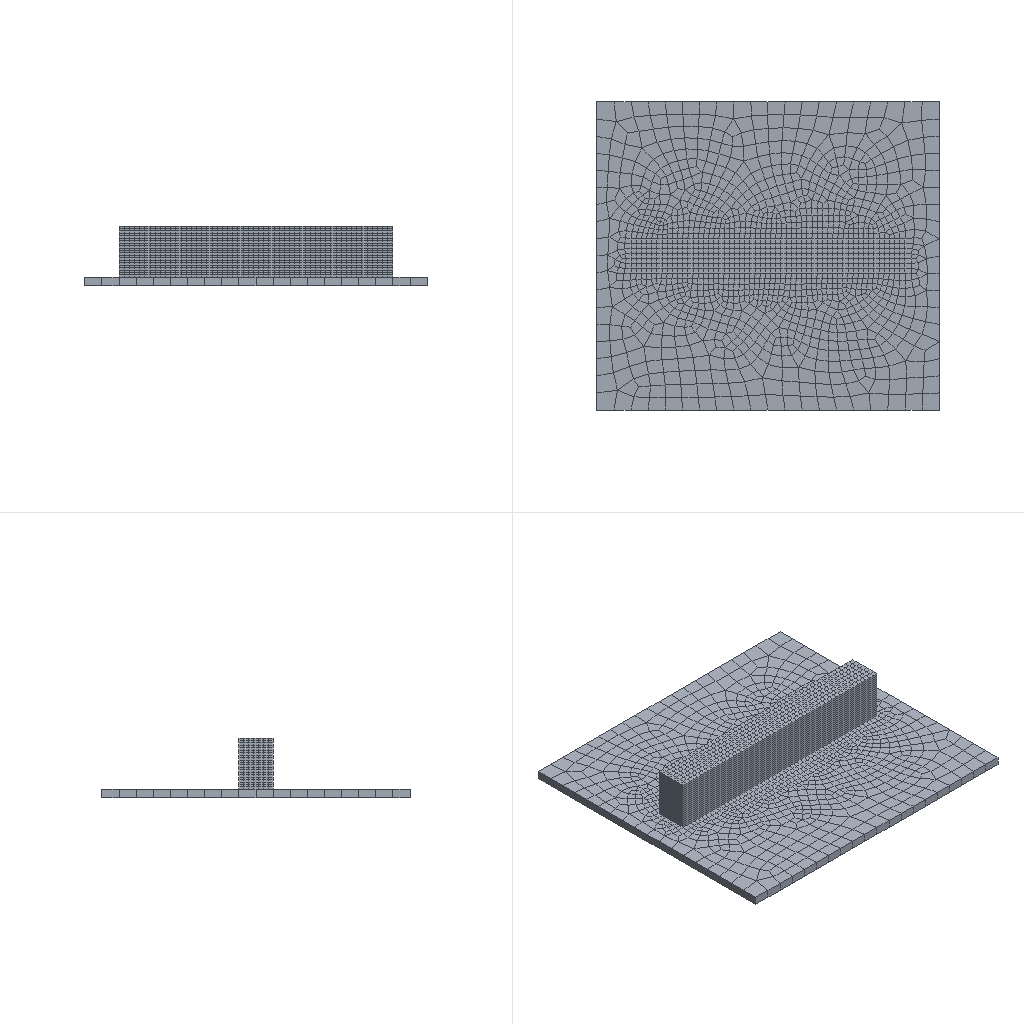Simulation study | abaqus
Abaqus input file, long lists of numbers shortened:
*Heading
** Job name: Job-1 Model name: Model-1
** Generated by: Abaqus/CAE 2017
*Preprint, echo=NO, model=NO, history=NO, contact=NO
**
** PARTS
**
*Part, name=Part-1
*Node
      1,          20.,        -100.,          15.
      2,         180.,        -100.,          15.
** (6268 more lines like these left out)
*Element, type=C3D8RT
   1,  260, 1113, 4399, 1041,    1,   17,  417,  132
   2, 1113, 1114, 4400, 4399,   17,   18,  418,  417
** (4179 more lines like these left out)
*Nset, nset=Set-8, generate
    1,  6270,     1
*Elset, elset=Set-8, generate
    1,  4181,     1
** Section: Section-1
*Solid Section, elset=Set-8, material=Material-1
,
*End Part
**
**
** ASSEMBLY
**
*Assembly, name=Assembly
**
*Instance, name=Part-1-1, part=Part-1
        -20.,          90.,         -15.
*End Instance
**
*Nset, nset=Set-1, instance=Part-1-1
   13,   14,   15,   16,  345,  346,  347,  348,  349,  350,  351,  352,  353,  354,  355,  356
  357,  358,  359,  360,  361,  362,  363,  364,  365,  366,  367,  368,  369,  370,  371,  372
** (100 more lines like these left out)
*Elset, elset=Set-1, instance=Part-1-1, generate
 2598,  4181,     1
*Nset, nset=Set-2, instance=Part-1-1, generate
    1,  6270,     1
*Elset, elset=Set-2, instance=Part-1-1, generate
    1,  4181,     1
*Nset, nset=Set-3, instance=Part-1-1
    1,    2,    3,    4,    5,    6,    7,    8,   17,   18,   19,   20,   21,   22,   23,   24
   25,   26,   27,   28,   29,   30,   31,   32,   33,   34,   35,   36,   37,   38,   39,   40
** (214 more lines like these left out)
*Elset, elset=Set-3, instance=Part-1-1, generate
    1,  2597,     1
*Nset, nset=Set-4, instance=Part-1-1
    1,    2,    3,    4,    5,    6,    7,    8,   17,   18,   19,   20,   21,   22,   23,   24
   25,   26,   27,   28,   29,   30,   31,   32,   33,   34,   35,   36,   37,   38,   39,   40
** (214 more lines like these left out)
*Elset, elset=Set-4, instance=Part-1-1, generate
    1,  2597,     1
*Nset, nset=Set-5, instance=Part-1-1
    1,    2,    3,    4,    5,    6,    7,    8,   17,   18,   19,   20,   21,   22,   23,   24
   25,   26,   27,   28,   29,   30,   31,   32,   33,   34,   35,   36,   37,   38,   39,   40
** (214 more lines like these left out)
*Elset, elset=Set-5, instance=Part-1-1, generate
    1,  2597,     1
*End Assembly
**
** MATERIALS
**
*Material, name=Material-1
*Conductivity
46.,
*Density
 7.8e-09,
*Elastic
206000., 0.3
*Expansion
 5e-06,
*Plastic
450.,0.
*Specific Heat
 4.6e+08,
** ----------------------------------------------------------------
**
** STEP: Step-1
**
*Step, name=Step-1, nlgeom=YES, inc=1000
*Coupled Temperature-displacement, creep=none, deltmx=1e+07, stabilize=0.0002, allsdtol=0.05, continue=NO
0.001, 0.01, 1e-07, 0.01
**
** BOUNDARY CONDITIONS
**
** Name: BC-1 Type: 对称/反对称/完全固定
*Boundary
Set-1, ENCASTRE
**
** INTERACTIONS
**
** Interaction: Int-1
*Model Change, remove
Set-3,
**
** OUTPUT REQUESTS
**
*Restart, write, frequency=0
**
** FIELD OUTPUT: F-Output-1
**
*Output, field
*Node Output
CF, NT, RF, RFL, RM, RT, U, V
*Element Output, directions=YES
ALPHAN, E, HFL, LE, MISES, MISESMAX, MISESONLY, PE, PEEQ, PEEQMAX, PEEQT, PEMAG, PEQC, PRESSONLY, S, SSAVG
TEMP
*Contact Output
CDISP, CSTRESS
*Radiation Output
FTEMP,
**
** HISTORY OUTPUT: H-Output-1
**
*Output, history, variable=PRESELECT
*End Step
** ----------------------------------------------------------------
**
** STEP: Step-2
**
*Step, name=Step-2, nlgeom=YES, inc=10000
*Coupled Temperature-displacement, creep=none, deltmx=1e+09, stabilize=0.0002, allsdtol=0.05, continue=NO
0.1, 10., 0.0001, 0.5
**
** LOADS
**
** Name: Load-1   Type: Body heat flux
*Dflux
Set-5, BFNU, 1.
**
** INTERACTIONS
**
** Interaction: Int-add
*Model Change, add
Set-4,
**
** OUTPUT REQUESTS
**
*Restart, write, frequency=0
**
** FIELD OUTPUT: F-Output-1
**
*Output, field
*Node Output
CF, NT, RF, RFL, RM, RT, U, V
*Element Output, directions=YES
ALPHAN, E, HFL, LE, MISES, MISESMAX, MISESONLY, PE, PEEQ, PEEQMAX, PEEQT, PEMAG, PEQC, PRESSONLY, S, SSAVG
TEMP
*Contact Output
CDISP, CSTRESS
*Radiation Output
FTEMP,
**
** HISTORY OUTPUT: H-Output-1
**
*Output, history, variable=PRESELECT
*End Step